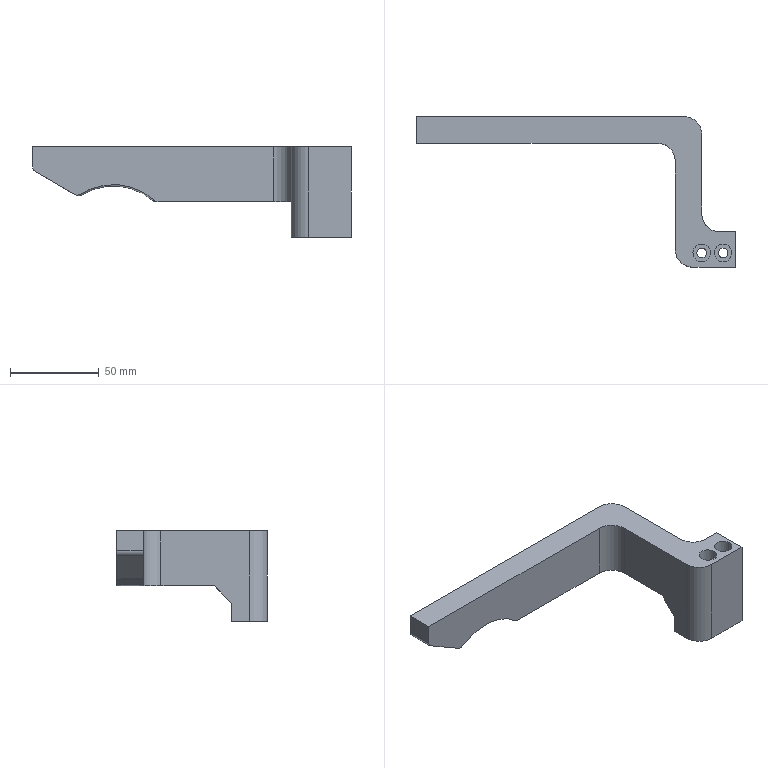NC program | NX | posted with a generic post | part box 180 x 85 x 51 mm
Lines 29210 to 29937 of 44959:
(FIXED_CONTOUR , TOOL : R4)
N58346 T08 M6
N58348 G54
N58350 G17 G0 G90 X-22.163 Y-24.602 S9500 M3
N58352 G43 Z30. H8
N58354 Z-16.099
N58356 G94 G1 X-22.13 Y-24.635 Z-16.62 F2500.
N58358 X-22.05 Y-24.715 Z-17.131
N58360 X-21.923 Y-24.842 Z-17.623
N58362 X-21.752 Y-25.013 Z-18.087
N58364 X-21.54 Y-25.225 Z-18.515
N58366 X-21.289 Y-25.476 Z-18.9
N58368 X-21.006 Y-25.759 Z-19.236
N58370 X-20.694 Y-26.071 Z-19.517
N58372 X-20.358 Y-26.407 Z-19.738
N58374 X-20.005 Y-26.76 Z-19.895
N58376 X-19.641 Y-27.124 Z-19.985
N58378 X-19.271 Y-27.494 Z-20.008
N58380 X-19.14 Y-27.625 Z-20.004
N58382 X-19.15 Y-27.75 Z-20.003
N58384 X-19.412 Y-27.487 Z-20.011
N58386 X-19.553 Y-27.481 Z-20.015
N58388 X-19.16 Y-27.875 Z-20.003
N58390 X-19.17 Y-27.999 Z-20.004
N58392 X-19.55 Y-27.619 Z-20.013
N58394 X-19.694 Y-27.475 Z-20.027
N58396 X-19.835 Y-27.468 Z-20.041
N58398 X-19.747 Y-27.556 Z-20.029
N58400 X-19.55 Y-27.753 Z-20.013
N58402 X-19.18 Y-28.124 Z-20.004
N58404 X-19.189 Y-28.249
N58406 X-19.55 Y-27.888 Z-20.012
N58408 X-19.813 Y-27.625 Z-20.033
N58410 X-19.976 Y-27.462 Z-20.055
N58412 X-20.117 Y-27.456 Z-20.071
N58414 X-19.833 Y-27.74 Z-20.034
N58416 X-19.55 Y-28.022 Z-20.012
N58418 X-19.199 Y-28.373 Z-20.003
N58420 X-19.209 Y-28.497
N58422 X-19.55 Y-28.156 Z-20.011
N58424 X-19.833 Y-27.874 Z-20.033
N58426 X-20.115 Y-27.591 Z-20.068
N58428 X-20.257 Y-27.45 Z-20.095
N58430 X-20.397 Y-27.443 Z-20.121
N58432 X-20.298 Y-27.542 Z-20.099
N58434 X-20.115 Y-27.725 Z-20.067
N58436 X-19.833 Y-28.007 Z-20.032
N58438 X-19.55 Y-28.29 Z-20.011
N58440 X-19.219 Y-28.621 Z-20.004
N58442 X-19.229 Y-28.745
N58444 X-19.55 Y-28.424 Z-20.01
N58446 X-19.833 Y-28.141 Z-20.03
N58448 X-20.115 Y-27.859 Z-20.065
N58450 X-20.365 Y-27.609 Z-20.109
N58452 X-20.537 Y-27.437 Z-20.147
N58454 X-20.677 Y-27.431 Z-20.175
N58456 X-20.398 Y-27.71 Z-20.113
N58458 X-20.115 Y-27.992 Z-20.064
N58460 X-19.833 Y-28.275 Z-20.029
N58462 X-19.55 Y-28.557 Z-20.01
N58464 X-19.238 Y-28.869 Z-20.004
N58466 X-19.248 Y-28.992
N58468 X-19.55 Y-28.69 Z-20.009
N58470 X-19.833 Y-28.407 Z-20.028
N58472 X-20.115 Y-28.125 Z-20.063
N58474 X-20.398 Y-27.842 Z-20.111
N58476 X-20.68 Y-27.56 Z-20.173
N58478 X-20.78 Y-27.46 Z-20.199
N58480 X-20.815 Y-27.425 Z-20.21
N58482 X-20.954 Y-27.419 Z-20.248
N58484 X-20.847 Y-27.526 Z-20.214
N58486 X-20.68 Y-27.692 Z-20.17
N58488 X-20.398 Y-27.975 Z-20.109
N58490 X-20.115 Y-28.257 Z-20.061
N58492 X-19.833 Y-28.54 Z-20.027
N58494 X-19.55 Y-28.822 Z-20.009
N58496 X-19.258 Y-29.115 Z-20.004
N58498 X-19.268 Y-29.238
N58500 X-19.55 Y-28.955 Z-20.008
N58502 X-19.833 Y-28.672 Z-20.026
N58504 X-20.115 Y-28.39 Z-20.06
N58506 X-20.398 Y-28.107 Z-20.107
N58508 X-20.68 Y-27.825 Z-20.168
N58510 X-20.914 Y-27.592 Z-20.229
N58512 X-21.093 Y-27.412 Z-20.285
N58514 X-21.232 Y-27.406 Z-20.324
N58516 X-20.963 Y-27.675 Z-20.239
N58518 X-20.68 Y-27.958 Z-20.166
N58520 X-20.398 Y-28.24 Z-20.106
N58522 X-20.115 Y-28.523 Z-20.059
N58524 X-19.833 Y-28.805 Z-20.026
N58526 X-19.55 Y-29.088 Z-20.008
N58528 X-19.277 Y-29.361 Z-20.003
N58530 X-19.287 Y-29.482 Z-20.004
N58532 X-19.55 Y-29.219 Z-20.007
N58534 X-19.833 Y-28.936 Z-20.025
N58536 X-20.115 Y-28.653 Z-20.057
N58538 X-20.398 Y-28.371 Z-20.104
N58540 X-20.68 Y-28.088 Z-20.163
N58542 X-20.963 Y-27.806 Z-20.236
N58544 X-21.245 Y-27.523 Z-20.325
N58546 X-21.327 Y-27.442 Z-20.355
N58548 X-21.369 Y-27.4 Z-20.372
N58550 X-21.505 Y-27.394 Z-20.422
N58552 X-21.392 Y-27.506 Z-20.375
N58554 X-21.245 Y-27.653 Z-20.321
N58556 X-20.963 Y-27.936 Z-20.233
N58558 X-20.68 Y-28.218 Z-20.161
N58560 X-20.398 Y-28.501 Z-20.103
N58562 X-20.115 Y-28.784 Z-20.056
N58564 X-19.833 Y-29.066 Z-20.024
N58566 X-19.55 Y-29.349 Z-20.007
N58568 X-19.296 Y-29.602 Z-20.004
N58570 X-19.306 Y-29.723 Z-20.003
N58572 X-19.55 Y-29.479 Z-20.006
N58574 X-19.833 Y-29.197 Z-20.023
N58576 X-20.115 Y-28.914 Z-20.055
N58578 X-20.398 Y-28.632 Z-20.101
N58580 X-20.68 Y-28.349 Z-20.159
N58582 X-20.963 Y-28.066 Z-20.231
N58584 X-21.245 Y-27.784 Z-20.318
N58586 X-21.458 Y-27.571 Z-20.396
N58588 X-21.642 Y-27.387 Z-20.472
N58590 X-21.779 Y-27.381 Z-20.522
N58592 X-21.524 Y-27.636 Z-20.417
N58594 X-21.245 Y-27.915 Z-20.315
N58596 X-20.962 Y-28.198 Z-20.228
N58598 X-20.68 Y-28.48 Z-20.156
N58600 X-20.398 Y-28.762 Z-20.099
N58602 X-20.115 Y-29.045 Z-20.054
N58604 X-19.833 Y-29.328 Z-20.022
N58606 X-19.55 Y-29.61 Z-20.006
N58608 X-19.316 Y-29.845 Z-20.003
N58610 X-19.325 Y-29.964
N58612 X-19.55 Y-29.739 Z-20.005
N58614 X-19.833 Y-29.456 Z-20.021
N58616 X-20.115 Y-29.174 Z-20.053
N58618 X-20.398 Y-28.891 Z-20.098
N58620 X-20.68 Y-28.609 Z-20.154
N58622 X-20.963 Y-28.326 Z-20.225
N58624 X-21.245 Y-28.043 Z-20.312
N58626 X-21.528 Y-27.761 Z-20.415
N58628 X-21.811 Y-27.478 Z-20.531
N58630 X-21.914 Y-27.375 Z-20.581
N58632 X-22.047 Y-27.369 Z-20.643
N58634 X-21.934 Y-27.483 Z-20.584
N58636 X-21.811 Y-27.606 Z-20.527
N58638 X-21.528 Y-27.888 Z-20.411
N58640 X-21.245 Y-28.171 Z-20.309
N58642 X-20.963 Y-28.454 Z-20.223
N58644 X-20.68 Y-28.736 Z-20.152
N58646 X-20.398 Y-29.019 Z-20.096
N58648 X-20.115 Y-29.301 Z-20.051
N58650 X-19.833 Y-29.584 Z-20.021
N58652 X-19.55 Y-29.866 Z-20.005
N58654 X-19.334 Y-30.082 Z-20.003
N58656 X-19.344 Y-30.201
N58658 X-19.55 Y-29.994 Z-20.004
N58660 X-19.833 Y-29.712 Z-20.02
N58662 X-20.115 Y-29.429 Z-20.05
N58664 X-20.398 Y-29.147 Z-20.094
N58666 X-20.68 Y-28.864 Z-20.15
N58668 X-20.963 Y-28.581 Z-20.22
N58670 X-21.245 Y-28.299 Z-20.306
N58672 X-21.528 Y-28.016 Z-20.408
N58674 X-21.811 Y-27.734 Z-20.522
N58676 X-21.998 Y-27.546 Z-20.611
N58678 X-22.093 Y-27.451 Z-20.66
N58680 X-22.181 Y-27.363 Z-20.709
N58682 X-22.315 Y-27.357 Z-20.775
N58684 X-22.062 Y-27.61 Z-20.637
N58686 X-21.811 Y-27.862 Z-20.518
N58688 X-21.528 Y-28.144 Z-20.404
N58690 X-21.245 Y-28.427 Z-20.303
N58692 X-20.963 Y-28.709 Z-20.217
N58694 X-20.68 Y-28.992 Z-20.148
N58696 X-20.358 Y-29.315 Z-20.086
N58698 X-20.115 Y-29.557 Z-20.049
N58700 X-19.833 Y-29.84 Z-20.019
N58702 X-19.55 Y-30.122 Z-20.004
N58704 X-19.353 Y-30.319 Z-20.002
N58706 X-19.362 Y-30.437
N58708 X-19.55 Y-30.249 Z-20.004
N58710 X-19.833 Y-29.967 Z-20.018
N58712 X-20.115 Y-29.684 Z-20.048
N58714 X-20.398 Y-29.401 Z-20.091
N58716 X-20.68 Y-29.119 Z-20.145
N58718 X-20.963 Y-28.836 Z-20.215
N58720 X-21.245 Y-28.554 Z-20.3
N58722 X-21.528 Y-28.271 Z-20.401
N58724 X-21.811 Y-27.989 Z-20.514
N58726 X-22.093 Y-27.706 Z-20.647
N58728 X-22.376 Y-27.424 Z-20.801
N58730 X-22.448 Y-27.351 Z-20.845
N58732 X-22.578 Y-27.345 Z-20.917
N58734 X-22.376 Y-27.548 Z-20.794
N58736 X-22.283 Y-27.64 Z-20.742
N58738 X-22.093 Y-27.83 Z-20.642
N58740 X-21.811 Y-28.113 Z-20.51
N58742 X-21.528 Y-28.395 Z-20.397
N58744 X-21.219 Y-28.704 Z-20.289
N58746 X-20.963 Y-28.96 Z-20.213
N58748 X-20.68 Y-29.243 Z-20.143
N58750 X-20.398 Y-29.525 Z-20.09
N58752 X-20.094 Y-29.83 Z-20.044
N58754 X-19.833 Y-30.091 Z-20.018
N58756 X-19.55 Y-30.373 Z-20.003
N58758 X-19.371 Y-30.552 Z-20.002
N58760 X-19.381 Y-30.667
N58762 X-19.573 Y-30.475 Z-20.004
N58764 X-19.833 Y-30.215 Z-20.017
N58766 X-20.115 Y-29.933 Z-20.046
N58768 X-20.398 Y-29.65 Z-20.088
N58770 X-20.698 Y-29.35 Z-20.145
N58772 X-20.963 Y-29.085 Z-20.21
N58774 X-21.245 Y-28.802 Z-20.294
N58776 X-21.528 Y-28.52 Z-20.394
N58778 X-21.811 Y-28.237 Z-20.506
N58780 X-22.093 Y-27.955 Z-20.638
N58782 X-22.376 Y-27.672 Z-20.787
N58784 X-22.658 Y-27.39 Z-20.958
N58786 X-22.708 Y-27.34 Z-20.992
N58788 X-22.838 Y-27.334 Z-21.072
N58790 X-22.658 Y-27.514 Z-20.95
N58792 X-22.532 Y-27.64 Z-20.873
N58794 X-22.376 Y-27.796 Z-20.782
N58796 X-22.093 Y-28.079 Z-20.634
N58798 X-21.811 Y-28.362 Z-20.502
N58800 X-21.528 Y-28.644 Z-20.39
N58802 X-21.245 Y-28.927 Z-20.291
N58804 X-20.963 Y-29.209 Z-20.208
N58806 X-20.68 Y-29.492 Z-20.139
N58808 X-20.398 Y-29.774 Z-20.086
N58810 X-20.115 Y-30.057 Z-20.045
N58812 X-19.802 Y-30.37 Z-20.015
N58814 X-19.55 Y-30.622 Z-20.003
N58816 X-19.39 Y-30.783 Z-20.002
N58818 X-19.399 Y-30.897
N58820 X-19.55 Y-30.746
N58822 X-19.833 Y-30.463 Z-20.016
N58824 X-20.115 Y-30.181 Z-20.044
N58826 X-20.398 Y-29.898 Z-20.085
N58828 X-20.68 Y-29.616 Z-20.137
N58830 X-20.963 Y-29.333 Z-20.205
N58832 X-21.245 Y-29.051 Z-20.289
N58834 X-21.528 Y-28.768 Z-20.387
N58836 X-21.811 Y-28.485 Z-20.499
N58838 X-22.093 Y-28.203 Z-20.629
N58840 X-22.376 Y-27.92 Z-20.777
N58842 X-22.657 Y-27.639 Z-20.942
N58844 X-22.941 Y-27.355 Z-21.133
N58846 X-22.968 Y-27.328 Z-21.153
N58848 X-23.093 Y-27.323 Z-21.238
N58850 X-22.941 Y-27.476 Z-21.125
N58852 X-22.776 Y-27.64 Z-21.014
N58854 X-22.658 Y-27.758 Z-20.937
N58856 X-22.376 Y-28.041 Z-20.772
N58858 X-22.093 Y-28.323 Z-20.625
N58860 X-21.811 Y-28.606 Z-20.495
N58862 X-21.528 Y-28.889 Z-20.384
N58864 X-21.245 Y-29.171 Z-20.286
N58866 X-20.963 Y-29.454 Z-20.203
N58868 X-20.68 Y-29.736 Z-20.135
N58870 X-20.398 Y-30.019 Z-20.083
N58872 X-20.115 Y-30.301 Z-20.042
N58874 X-19.833 Y-30.584 Z-20.015
N58876 X-19.55 Y-30.866 Z-20.002
N58878 X-19.408 Y-31.009 Z-20.001
N58880 X-19.416 Y-31.121
N58882 X-19.549 Y-30.989 Z-20.002
N58884 X-19.833 Y-30.705 Z-20.015
N58886 X-20.115 Y-30.422 Z-20.041
N58888 X-20.398 Y-30.14 Z-20.082
N58890 X-20.68 Y-29.857 Z-20.133
N58892 X-20.963 Y-29.575 Z-20.201
N58894 X-21.245 Y-29.292 Z-20.283
N58896 X-21.528 Y-29.01 Z-20.38
N58898 X-21.811 Y-28.727 Z-20.491
N58900 X-22.093 Y-28.444 Z-20.621
N58902 X-22.376 Y-28.162 Z-20.767
N58904 X-22.658 Y-27.879 Z-20.931
N58906 X-22.941 Y-27.597 Z-21.116
N58908 X-23.219 Y-27.318 Z-21.325
N58910 X-23.345 Y-27.313 Z-21.42
N58912 X-23.223 Y-27.435 Z-21.319
N58914 X-22.941 Y-27.717 Z-21.11
N58916 X-22.658 Y-28. Z-20.926
N58918 X-22.376 Y-28.282 Z-20.762
N58920 X-22.093 Y-28.565 Z-20.616
N58922 X-21.811 Y-28.847 Z-20.487
N58924 X-21.528 Y-29.13 Z-20.377
N58926 X-21.245 Y-29.412 Z-20.28
N58928 X-20.963 Y-29.695 Z-20.198
N58930 X-20.68 Y-29.978 Z-20.131
N58932 X-20.398 Y-30.26 Z-20.08
N58934 X-20.115 Y-30.543 Z-20.04
N58936 X-19.833 Y-30.825 Z-20.014
N58938 X-19.55 Y-31.108 Z-20.002
N58940 X-19.425 Y-31.233 Z-20.001
N58942 X-19.434 Y-31.344
N58944 X-19.55 Y-31.228
N58946 X-19.833 Y-30.945 Z-20.014
N58948 X-20.115 Y-30.663 Z-20.039
N58950 X-20.398 Y-30.38 Z-20.079
N58952 X-20.68 Y-30.098 Z-20.13
N58954 X-20.963 Y-29.815 Z-20.196
N58956 X-21.245 Y-29.532 Z-20.278
N58958 X-21.528 Y-29.25 Z-20.374
N58960 X-21.811 Y-28.967 Z-20.483
N58962 X-22.093 Y-28.685 Z-20.612
N58964 X-22.376 Y-28.402 Z-20.757
N58966 X-22.658 Y-28.12 Z-20.92
N58968 X-22.941 Y-27.837 Z-21.103
N58970 X-23.223 Y-27.555 Z-21.31
N58972 X-23.469 Y-27.309 Z-21.515
N58974 X-23.506 Y-27.307 Z-21.542
N58976 X-23.59 Y-27.304 Z-21.614
N58978 X-23.506 Y-27.388 Z-21.536
N58980 X-23.223 Y-27.671 Z-21.302
N58982 X-22.941 Y-27.953 Z-21.098
N58984 X-22.658 Y-28.236 Z-20.915
N58986 X-22.376 Y-28.518 Z-20.752
N58988 X-22.093 Y-28.801 Z-20.608
N58990 X-21.811 Y-29.083 Z-20.48
N58992 X-21.528 Y-29.366 Z-20.371
N58994 X-21.245 Y-29.649 Z-20.275
N58996 X-20.963 Y-29.931 Z-20.194
N58998 X-20.68 Y-30.214 Z-20.128
N59000 X-20.398 Y-30.496 Z-20.077
N59002 X-20.115 Y-30.779 Z-20.038
N59004 X-19.833 Y-31.061 Z-20.013
N59006 X-19.55 Y-31.344 Z-20.001
N59008 X-19.443 Y-31.451
N59010 X-19.451 Y-31.558
N59012 X-19.55 Y-31.459
N59014 X-19.833 Y-31.176 Z-20.013
N59016 X-20.115 Y-30.894 Z-20.037
N59018 X-20.398 Y-30.611 Z-20.076
N59020 X-20.68 Y-30.328 Z-20.126
N59022 X-20.963 Y-30.046 Z-20.192
N59024 X-21.245 Y-29.763 Z-20.272
N59026 X-21.528 Y-29.481 Z-20.367
N59028 X-21.811 Y-29.198 Z-20.476
N59030 X-22.093 Y-28.916 Z-20.604
N59032 X-22.376 Y-28.633 Z-20.747
N59034 X-22.658 Y-28.351 Z-20.91
N59036 X-22.941 Y-28.068 Z-21.092
N59038 X-23.223 Y-27.785 Z-21.296
N59040 X-23.369 Y-27.64 Z-21.413
N59042 X-23.506 Y-27.503 Z-21.527
N59044 X-23.707 Y-27.302 Z-21.714
N59046 X-23.823 Y-27.3 Z-21.814
N59048 X-23.506 Y-27.617 Z-21.518
N59050 X-23.223 Y-27.899 Z-21.29
N59052 X-22.941 Y-28.182 Z-21.086
N59054 X-22.658 Y-28.464 Z-20.905
N59056 X-22.376 Y-28.747 Z-20.743
N59058 X-22.093 Y-29.029 Z-20.6
N59060 X-21.811 Y-29.312 Z-20.473
N59062 X-21.528 Y-29.595 Z-20.364
N59064 X-21.245 Y-29.877 Z-20.27
N59066 X-20.963 Y-30.16 Z-20.19
N59068 X-20.68 Y-30.442 Z-20.124
N59070 X-20.398 Y-30.725 Z-20.074
N59072 X-20.115 Y-31.007 Z-20.036
N59074 X-19.833 Y-31.29 Z-20.013
N59076 X-19.55 Y-31.572 Z-20.001
N59078 X-19.459 Y-31.663
N59080 X-19.468 Y-31.768
N59082 X-19.597 Y-31.639 Z-20.002
N59084 X-19.833 Y-31.403 Z-20.012
N59086 X-20.115 Y-31.12 Z-20.035
N59088 X-20.398 Y-30.838 Z-20.073
N59090 X-20.68 Y-30.555 Z-20.123
N59092 X-20.963 Y-30.273 Z-20.188
N59094 X-21.245 Y-29.99 Z-20.267
N59096 X-21.528 Y-29.708 Z-20.361
N59098 X-21.811 Y-29.425 Z-20.469
N59100 X-22.093 Y-29.142 Z-20.596
N59102 X-22.376 Y-28.86 Z-20.738
N59104 X-22.658 Y-28.577 Z-20.9
N59106 X-22.941 Y-28.295 Z-21.08
N59108 X-23.223 Y-28.012 Z-21.283
N59110 X-23.506 Y-27.73 Z-21.511
N59112 X-23.938 Y-27.297 Z-21.912
N59114 X-24.053 Y-27.295 Z-22.009
N59116 X-23.574 Y-27.774 Z-21.564
N59118 X-23.506 Y-27.842 Z-21.504
N59120 X-23.223 Y-28.124 Z-21.277
N59122 X-22.941 Y-28.407 Z-21.075
N59124 X-22.658 Y-28.69 Z-20.895
N59126 X-22.376 Y-28.972 Z-20.734
N59128 X-22.093 Y-29.255 Z-20.592
N59130 X-21.811 Y-29.537 Z-20.466
N59132 X-21.528 Y-29.82 Z-20.358
N59134 X-21.245 Y-30.102 Z-20.264
N59136 X-20.963 Y-30.385 Z-20.186
N59138 X-20.68 Y-30.667 Z-20.121
N59140 X-20.398 Y-30.95 Z-20.072
N59142 X-20.115 Y-31.233 Z-20.034
N59144 X-19.833 Y-31.515 Z-20.012
N59146 X-19.55 Y-31.798 Z-20.001
N59148 X-19.476 Y-31.872
N59150 X-19.484 Y-31.975 Z-20.
N59152 X-19.55 Y-31.909 Z-20.001
N59154 X-19.833 Y-31.626 Z-20.011
N59156 X-20.115 Y-31.344 Z-20.033
N59158 X-20.422 Y-31.037 Z-20.074
N59160 X-20.68 Y-30.779 Z-20.119
N59162 X-20.963 Y-30.496 Z-20.184
N59164 X-21.245 Y-30.213 Z-20.262
N59166 X-21.548 Y-29.911 Z-20.362
N59168 X-21.811 Y-29.648 Z-20.462
N59170 X-22.093 Y-29.366 Z-20.588
N59172 X-22.376 Y-29.083 Z-20.729
N59174 X-22.658 Y-28.801 Z-20.89
N59176 X-22.941 Y-28.518 Z-21.069
N59178 X-23.223 Y-28.236 Z-21.271
N59180 X-23.506 Y-27.953 Z-21.497
N59182 X-23.611 Y-27.848 Z-21.59
N59184 X-24.166 Y-27.293 Z-22.107
N59186 X-24.277 Z-22.203
N59188 X-23.93 Y-27.64 Z-21.877
N59190 X-23.648 Y-27.922 Z-21.616
N59192 X-23.506 Y-28.064 Z-21.49
N59194 X-23.223 Y-28.346 Z-21.265
N59196 X-22.941 Y-28.629 Z-21.064
N59198 X-22.658 Y-28.912 Z-20.885
N59200 X-22.376 Y-29.194 Z-20.725
N59202 X-22.093 Y-29.477 Z-20.584
N59204 X-21.811 Y-29.759 Z-20.459
N59206 X-21.528 Y-30.042 Z-20.352
N59208 X-21.245 Y-30.324 Z-20.259
N59210 X-20.963 Y-30.607 Z-20.182
N59212 X-20.68 Y-30.889 Z-20.118
N59214 X-20.398 Y-31.172 Z-20.069
N59216 X-20.115 Y-31.455 Z-20.032
N59218 X-19.833 Y-31.737 Z-20.011
N59220 X-19.55 Y-32.02 Z-20.
N59222 X-19.492 Y-32.078
N59224 X-19.5 Y-32.18
N59226 X-19.55 Y-32.13
N59228 X-19.833 Y-31.848 Z-20.011
N59230 X-20.115 Y-31.565 Z-20.031
N59232 X-20.398 Y-31.283 Z-20.068
N59234 X-20.68 Y-31. Z-20.116
N59236 X-20.963 Y-30.717 Z-20.18
N59238 X-21.245 Y-30.435 Z-20.257
N59240 X-21.528 Y-30.152 Z-20.349
N59242 X-21.81 Y-29.871 Z-20.455
N59244 X-22.093 Y-29.587 Z-20.58
N59246 X-22.376 Y-29.305 Z-20.72
N59248 X-22.658 Y-29.022 Z-20.88
N59250 X-22.941 Y-28.74 Z-21.058
N59252 X-23.223 Y-28.457 Z-21.259
N59254 X-23.506 Y-28.174 Z-21.484
N59256 X-23.685 Y-27.995 Z-21.643
N59258 X-24.071 Y-27.609 Z-21.999
N59260 X-24.388 Y-27.292 Z-22.299
N59262 X-24.499 Z-22.395
N59264 X-24.15 Y-27.64 Z-22.065
N59266 X-23.723 Y-28.068 Z-21.669
N59268 X-23.506 Y-28.285 Z-21.477
N59270 X-23.223 Y-28.567 Z-21.253
N59272 X-22.941 Y-28.85 Z-21.053
N59274 X-22.658 Y-29.132 Z-20.875
N59276 X-22.376 Y-29.415 Z-20.716
N59278 X-22.093 Y-29.698 Z-20.576
N59280 X-21.811 Y-29.98 Z-20.452
N59282 X-21.528 Y-30.263 Z-20.346
N59284 X-21.245 Y-30.545 Z-20.254
N59286 X-20.963 Y-30.828 Z-20.178
N59288 X-20.68 Y-31.11 Z-20.115
N59290 X-20.398 Y-31.393 Z-20.067
N59292 X-20.115 Y-31.675 Z-20.031
N59294 X-19.833 Y-31.958 Z-20.01
N59296 X-19.55 Y-32.241 Z-20.
N59298 X-19.508 Y-32.282
N59300 X-19.516 Y-32.384
N59302 X-19.833 Y-32.068 Z-20.01
N59304 X-20.115 Y-31.785 Z-20.03
N59306 X-20.398 Y-31.503 Z-20.065
N59308 X-20.68 Y-31.22 Z-20.113
N59310 X-20.963 Y-30.938 Z-20.176
N59312 X-21.245 Y-30.655 Z-20.252
N59314 X-21.528 Y-30.373 Z-20.343
N59316 X-21.811 Y-30.09 Z-20.449
N59318 X-22.093 Y-29.807 Z-20.572
N59320 X-22.376 Y-29.525 Z-20.712
N59322 X-22.658 Y-29.242 Z-20.87
N59324 X-22.941 Y-28.96 Z-21.048
N59326 X-23.223 Y-28.677 Z-21.247
N59328 X-23.506 Y-28.395 Z-21.47
N59330 X-23.759 Y-28.141 Z-21.695
N59332 X-24.26 Y-27.64 Z-22.16
N59334 X-24.609 Y-27.292 Z-22.49
N59336 X-24.722 Y-27.291 Z-22.582
N59338 X-24.636 Y-27.377 Z-22.507
N59340 X-24.373 Y-27.64 Z-22.257
N59342 X-23.762 Y-28.251 Z-21.69
N59344 X-23.506 Y-28.507 Z-21.464
N59346 X-23.223 Y-28.789 Z-21.241
N59348 X-22.941 Y-29.072 Z-21.042
N59350 X-22.658 Y-29.355 Z-20.865
N59352 X-22.376 Y-29.637 Z-20.707
N59354 X-22.093 Y-29.92 Z-20.568
N59356 X-21.811 Y-30.202 Z-20.446
N59358 X-21.528 Y-30.485 Z-20.34
N59360 X-21.245 Y-30.767 Z-20.249
N59362 X-20.963 Y-31.05 Z-20.174
N59364 X-20.68 Y-31.332 Z-20.112
N59366 X-20.398 Y-31.615 Z-20.064
N59368 X-20.115 Y-31.898 Z-20.029
N59370 X-19.833 Y-32.18 Z-20.01
N59372 X-19.524 Y-32.488 Z-20.
N59374 X-19.533 Y-32.595
N59376 X-19.833 Y-32.296 Z-20.009
N59378 X-20.115 Y-32.013 Z-20.028
N59380 X-20.398 Y-31.731 Z-20.063
N59382 X-20.68 Y-31.448 Z-20.11
N59384 X-20.963 Y-31.165 Z-20.172
N59386 X-21.245 Y-30.883 Z-20.247
N59388 X-21.528 Y-30.6 Z-20.337
N59390 X-21.811 Y-30.318 Z-20.443
N59392 X-22.093 Y-30.035 Z-20.564
N59394 X-22.376 Y-29.753 Z-20.703
N59396 X-22.658 Y-29.47 Z-20.86
N59398 X-22.941 Y-29.188 Z-21.037
N59400 X-23.223 Y-28.905 Z-21.235
N59402 X-23.506 Y-28.622 Z-21.457
N59404 X-23.788 Y-28.34 Z-21.705
N59406 X-24.488 Y-27.64 Z-22.357
N59408 X-24.636 Y-27.492 Z-22.497
N59410 X-24.837 Y-27.291 Z-22.675
N59412 X-24.956 Z-22.77
N59414 X-24.636 Y-27.611 Z-22.487
N59416 X-23.788 Y-28.459 Z-21.697
N59418 X-23.506 Y-28.741 Z-21.45
N59420 X-23.223 Y-29.024 Z-21.228
N59422 X-22.941 Y-29.306 Z-21.031
N59424 X-22.658 Y-29.589 Z-20.855
N59426 X-22.375 Y-29.873 Z-20.698
N59428 X-22.093 Y-30.154 Z-20.56
N59430 X-21.811 Y-30.437 Z-20.439
N59432 X-21.528 Y-30.719 Z-20.334
N59434 X-21.245 Y-31.002 Z-20.244
N59436 X-20.963 Y-31.284 Z-20.17
N59438 X-20.68 Y-31.567 Z-20.108
N59440 X-20.398 Y-31.849 Z-20.062
N59442 X-20.115 Y-32.132 Z-20.027
N59444 X-19.833 Y-32.415 Z-20.009
N59446 X-19.542 Y-32.706 Z-20.
N59448 X-19.55 Y-32.815
N59450 X-19.833 Y-32.532 Z-20.009
N59452 X-20.115 Y-32.25 Z-20.026
N59454 X-20.398 Y-31.967 Z-20.06
N59456 X-20.68 Y-31.685 Z-20.107
N59458 X-20.963 Y-31.402 Z-20.168
N59460 X-21.245 Y-31.12 Z-20.241
N59462 X-21.528 Y-30.837 Z-20.331
N59464 X-21.811 Y-30.554 Z-20.436
N59466 X-22.093 Y-30.272 Z-20.556
N59468 X-22.376 Y-29.989 Z-20.694
N59470 X-22.658 Y-29.707 Z-20.85
N59472 X-22.941 Y-29.424 Z-21.025
N59474 X-23.223 Y-29.142 Z-21.222
N59476 X-23.506 Y-28.859 Z-21.442
N59478 X-23.788 Y-28.577 Z-21.69
N59480 X-24.636 Y-27.729 Z-22.479
N59482 X-25.074 Y-27.291 Z-22.865
N59484 X-25.191 Z-22.959
N59486 X-24.636 Y-27.846 Z-22.471
N59488 X-23.788 Y-28.694 Z-21.682
N59490 X-23.506 Y-28.976 Z-21.435
N59492 X-23.223 Y-29.259 Z-21.216
N59494 X-22.941 Y-29.541 Z-21.02
N59496 X-22.658 Y-29.824 Z-20.845
N59498 X-22.376 Y-30.107 Z-20.689
N59500 X-22.093 Y-30.389 Z-20.552
N59502 X-21.811 Y-30.672 Z-20.432
N59504 X-21.528 Y-30.954 Z-20.328
N59506 X-21.245 Y-31.237 Z-20.239
N59508 X-20.935 Y-31.547 Z-20.16
N59510 X-20.68 Y-31.802 Z-20.105
N59512 X-20.398 Y-32.084 Z-20.059
N59514 X-20.115 Y-32.367 Z-20.026
N59516 X-19.833 Y-32.65 Z-20.008
N59518 X-19.559 Y-32.923 Z-20.
N59520 X-19.567 Y-33.032
N59522 X-19.833 Y-32.767 Z-20.008
N59524 X-20.115 Y-32.484 Z-20.025
N59526 X-20.43 Y-32.169 Z-20.063
N59528 X-20.68 Y-31.919 Z-20.104
N59530 X-20.993 Y-31.606 Z-20.172
N59532 X-21.245 Y-31.354 Z-20.236
N59534 X-21.556 Y-31.044 Z-20.335
N59536 X-21.811 Y-30.789 Z-20.429
N59538 X-22.093 Y-30.506 Z-20.548
N59540 X-22.376 Y-30.224 Z-20.685
N59542 X-22.658 Y-29.941 Z-20.84
N59544 X-22.941 Y-29.659 Z-21.014
N59546 X-23.223 Y-29.376 Z-21.21
N59548 X-23.506 Y-29.093 Z-21.428
N59550 X-23.788 Y-28.811 Z-21.674
N59552 X-24.636 Y-27.963 Z-22.463
N59554 X-25.059 Y-27.54 Z-22.833
N59556 X-25.308 Y-27.291 Z-23.052
N59558 X-25.425 Z-23.144
N59560 X-24.636 Y-28.08 Z-22.455
N59562 X-23.788 Y-28.928 Z-21.666
N59564 X-23.506 Y-29.211 Z-21.421
N59566 X-23.223 Y-29.493 Z-21.204
N59568 X-22.941 Y-29.776 Z-21.009
N59570 X-22.658 Y-30.058 Z-20.835
N59572 X-22.376 Y-30.341 Z-20.68
N59574 X-22.093 Y-30.623 Z-20.544
N59576 X-21.783 Y-30.934 Z-20.415
N59578 X-21.528 Y-31.188 Z-20.323
N59580 X-21.245 Y-31.471 Z-20.234
N59582 X-20.963 Y-31.754 Z-20.162
N59584 X-20.657 Y-32.059 Z-20.098
N59586 X-20.398 Y-32.319 Z-20.057
N59588 X-20.115 Y-32.601 Z-20.024
N59590 X-19.833 Y-32.884 Z-20.008
N59592 X-19.576 Y-33.141 Z-20.001
N59594 X-19.585 Y-33.249
N59596 X-19.833 Y-33.001 Z-20.007
N59598 X-20.115 Y-32.718 Z-20.023
N59600 X-20.398 Y-32.436 Z-20.056
N59602 X-20.68 Y-32.153 Z-20.101
N59604 X-20.963 Y-31.871 Z-20.16
N59606 X-21.245 Y-31.588 Z-20.231
N59608 X-21.528 Y-31.306 Z-20.32
N59610 X-21.811 Y-31.023 Z-20.422
N59612 X-22.093 Y-30.74 Z-20.541
N59614 X-22.376 Y-30.458 Z-20.676
N59616 X-22.658 Y-30.175 Z-20.83
N59618 X-22.941 Y-29.893 Z-21.003
N59620 X-23.223 Y-29.61 Z-21.198
N59622 X-23.506 Y-29.328 Z-21.414
N59624 X-23.788 Y-29.045 Z-21.658
N59626 X-24.635 Y-28.198 Z-22.446
N59628 X-25.542 Y-27.291 Z-23.237
N59630 X-25.66 Z-23.33
N59632 X-24.636 Y-28.315 Z-22.439
N59634 X-23.788 Y-29.162 Z-21.65
N59636 X-23.506 Y-29.445 Z-21.407
N59638 X-23.223 Y-29.727 Z-21.191
N59640 X-22.941 Y-30.01 Z-20.998
N59642 X-22.658 Y-30.292 Z-20.825
N59644 X-22.376 Y-30.575 Z-20.672
N59646 X-22.093 Y-30.858 Z-20.537
N59648 X-21.811 Y-31.14 Z-20.419
N59650 X-21.528 Y-31.423 Z-20.317
N59652 X-21.245 Y-31.705 Z-20.229
N59654 X-20.963 Y-31.988 Z-20.158
N59656 X-20.68 Y-32.27 Z-20.099
N59658 X-20.398 Y-32.553 Z-20.054
N59660 X-20.115 Y-32.835 Z-20.022
N59662 X-19.79 Y-33.16 Z-20.006
N59664 X-19.593 Y-33.358 Z-20.001
N59666 X-19.602 Y-33.466
N59668 X-19.837 Y-33.231 Z-20.007
N59670 X-20.115 Y-32.953 Z-20.022
N59672 X-20.398 Y-32.67 Z-20.053
N59674 X-20.68 Y-32.388 Z-20.098
N59676 X-20.963 Y-32.105 Z-20.156
N59678 X-21.245 Y-31.823 Z-20.227
N59680 X-21.528 Y-31.54 Z-20.314
N59682 X-21.811 Y-31.257 Z-20.416
N59684 X-22.093 Y-30.975 Z-20.533
N59686 X-22.376 Y-30.692 Z-20.667
N59688 X-22.658 Y-30.41 Z-20.821
N59690 X-22.941 Y-30.127 Z-20.992
N59692 X-23.223 Y-29.845 Z-21.185
N59694 X-23.506 Y-29.562 Z-21.4
N59696 X-23.788 Y-29.28 Z-21.642
N59698 X-24.636 Y-28.432 Z-22.431
N59700 X-25.201 Y-27.867 Z-22.924
N59702 X-25.428 Y-27.64 Z-23.118
N59704 X-25.777 Y-27.291 Z-23.422
N59706 X-25.898 Z-23.51
N59708 X-25.766 Y-27.422 Z-23.404
N59710 X-25.548 Y-27.64 Z-23.214
N59712 X-25.201 Y-27.987 Z-22.916
N59714 X-24.636 Y-28.553 Z-22.423
N59716 X-23.788 Y-29.4 Z-21.634
N59718 X-23.506 Y-29.683 Z-21.393
N59720 X-23.223 Y-29.965 Z-21.179
N59722 X-22.941 Y-30.248 Z-20.987
N59724 X-22.658 Y-30.53 Z-20.816
N59726 X-22.376 Y-30.813 Z-20.663
N59728 X-22.093 Y-31.096 Z-20.529
N59730 X-21.811 Y-31.378 Z-20.413
N59732 X-21.528 Y-31.661 Z-20.311
N59734 X-21.245 Y-31.943 Z-20.224
N59736 X-20.963 Y-32.226 Z-20.154
N59738 X-20.68 Y-32.508 Z-20.097
N59740 X-20.398 Y-32.791 Z-20.052
N59742 X-20.115 Y-33.073 Z-20.021
N59744 X-19.878 Y-33.311 Z-20.008
N59746 X-19.61 Y-33.578 Z-20.001
N59748 X-19.619 Y-33.69 Z-20.002
N59750 X-19.919 Y-33.391 Z-20.01
N59752 X-20.115 Y-33.194 Z-20.02
N59754 X-20.398 Y-32.912 Z-20.051
N59756 X-20.68 Y-32.629 Z-20.095
N59758 X-20.963 Y-32.346 Z-20.152
N59760 X-21.245 Y-32.064 Z-20.222
N59762 X-21.528 Y-31.781 Z-20.308
N59764 X-21.811 Y-31.499 Z-20.409
N59766 X-22.093 Y-31.216 Z-20.525
N59768 X-22.376 Y-30.934 Z-20.658
N59770 X-22.658 Y-30.651 Z-20.811
N59772 X-22.941 Y-30.369 Z-20.981
N59774 X-23.223 Y-30.086 Z-21.173
N59776 X-23.506 Y-29.803 Z-21.386
N59778 X-23.788 Y-29.521 Z-21.626
N59780 X-24.636 Y-28.673 Z-22.415
N59782 X-25.201 Y-28.108 Z-22.908
N59784 X-25.766 Y-27.543 Z-23.394
N59786 X-26.018 Y-27.291 Z-23.598
N59788 X-26.138 Z-23.686
N59790 X-25.766 Y-27.663 Z-23.385
N59792 X-25.201 Y-28.228 Z-22.9
N59794 X-24.636 Y-28.793 Z-22.406